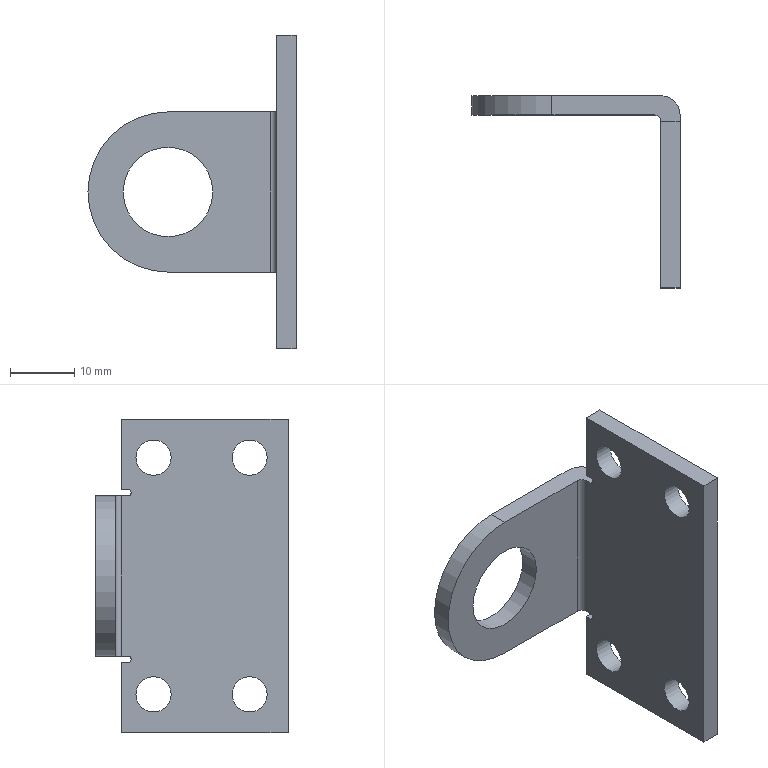Part | NX | features 5003_213_Bracket 2 | 1 solid | 23 faces | box 32.5 x 30 x 49 mm | volume 5335 mm3 | plane 13 | cylinder 10 | commonest cylinder face diameters 5.5 x4 1 x2 2 x1 6 x1 14 x1 25 x1
STEP:
#1=CARTESIAN_POINT('',(-223.775,-557.1,-110.5));
#2=VERTEX_POINT('',#1);
#3=CARTESIAN_POINT('',(-216.775,-557.1,-110.5));
#4=DIRECTION('',(0.,1.,0.));
#5=DIRECTION('',(-1.,0.,0.));
#6=AXIS2_PLACEMENT_3D('',#3,#4,#5);
#7=CIRCLE('',#6,7.);
#8=EDGE_CURVE('',#2,#2,#7,.T.);
#9=ORIENTED_EDGE('',*,*,#8,.T.);
#10=EDGE_LOOP('',(#9));
#11=FACE_BOUND('',#10,.T.);
#12=CARTESIAN_POINT('',(-200.775,-557.1,-123.));
#13=VERTEX_POINT('',#12);
#14=CARTESIAN_POINT('',(-216.775,-557.1,-123.));
#15=VERTEX_POINT('',#14);
#16=CARTESIAN_POINT('',(-216.775,-557.1,-123.));
#17=DIRECTION('',(-1.,0.,0.));
#18=VECTOR('',#17,1000.);
#19=LINE('',#16,#18);
#20=EDGE_CURVE('',#13,#15,#19,.T.);
#21=ORIENTED_EDGE('',*,*,#20,.F.);
#22=CARTESIAN_POINT('',(-200.775,-557.1,-98.));
#23=VERTEX_POINT('',#22);
#24=CARTESIAN_POINT('',(-200.775,-557.1,-98.));
#25=DIRECTION('',(0.,0.,-1.));
#26=VECTOR('',#25,1000.);
#27=LINE('',#24,#26);
#28=EDGE_CURVE('',#13,#23,#27,.F.);
#29=ORIENTED_EDGE('',*,*,#28,.T.);
#30=CARTESIAN_POINT('',(-216.775,-557.1,-98.));
#31=VERTEX_POINT('',#30);
#32=CARTESIAN_POINT('',(-216.775,-557.1,-98.));
#33=DIRECTION('',(1.,0.,0.));
#34=VECTOR('',#33,1000.);
#35=LINE('',#32,#34);
#36=EDGE_CURVE('',#31,#23,#35,.T.);
#37=ORIENTED_EDGE('',*,*,#36,.F.);
#38=CARTESIAN_POINT('',(-216.775,-557.1,-110.5));
#39=DIRECTION('',(0.,1.,0.));
#40=DIRECTION('',(-1.,0.,0.));
#41=AXIS2_PLACEMENT_3D('',#38,#39,#40);
#42=CIRCLE('',#41,12.5);
#43=EDGE_CURVE('',#15,#31,#42,.T.);
#44=ORIENTED_EDGE('',*,*,#43,.F.);
#45=EDGE_LOOP('',(#21,#29,#37,#44));
#46=FACE_BOUND('',#45,.T.);
#47=CARTESIAN_POINT('',(-216.775,-557.1,-110.5));
#48=DIRECTION('',(0.,1.,0.));
#49=DIRECTION('',(-1.,0.,0.));
#50=AXIS2_PLACEMENT_3D('',#47,#48,#49);
#51=PLANE('',#50);
#52=ADVANCED_FACE('',(#11,#46),#51,.F.);
#53=ORIENTED_EDGE('',*,*,#36,.T.);
#54=CARTESIAN_POINT('',(-199.775,-558.1,-98.));
#55=VERTEX_POINT('',#54);
#56=CARTESIAN_POINT('',(-200.775,-558.1,-98.));
#57=DIRECTION('',(0.,0.,-1.));
#58=DIRECTION('',(0.,-1.,0.));
#59=AXIS2_PLACEMENT_3D('',#56,#57,#58);
#60=CIRCLE('',#59,1.);
#61=EDGE_CURVE('',#23,#55,#60,.T.);
#62=ORIENTED_EDGE('',*,*,#61,.T.);
#63=CARTESIAN_POINT('',(-199.775,-559.1,-98.));
#64=VERTEX_POINT('',#63);
#65=CARTESIAN_POINT('',(-199.775,-584.1,-98.));
#66=DIRECTION('',(0.,1.,0.));
#67=VECTOR('',#66,1000.);
#68=LINE('',#65,#67);
#69=EDGE_CURVE('',#64,#55,#68,.T.);
#70=ORIENTED_EDGE('',*,*,#69,.F.);
#71=CARTESIAN_POINT('',(-196.775,-559.1,-98.));
#72=VERTEX_POINT('',#71);
#73=CARTESIAN_POINT('',(-229.275,-559.1,-98.));
#74=DIRECTION('',(1.,0.,0.));
#75=VECTOR('',#74,1000.);
#76=LINE('',#73,#75);
#77=EDGE_CURVE('',#64,#72,#76,.T.);
#78=ORIENTED_EDGE('',*,*,#77,.T.);
#79=CARTESIAN_POINT('',(-196.775,-557.1,-98.));
#80=VERTEX_POINT('',#79);
#81=CARTESIAN_POINT('',(-196.775,-554.1,-98.));
#82=DIRECTION('',(0.,-1.,0.));
#83=VECTOR('',#82,1000.);
#84=LINE('',#81,#83);
#85=EDGE_CURVE('',#80,#72,#84,.T.);
#86=ORIENTED_EDGE('',*,*,#85,.F.);
#87=CARTESIAN_POINT('',(-199.775,-554.1,-98.));
#88=VERTEX_POINT('',#87);
#89=CARTESIAN_POINT('',(-199.775,-557.1,-98.));
#90=DIRECTION('',(0.,0.,-1.));
#91=DIRECTION('',(0.,-1.,0.));
#92=AXIS2_PLACEMENT_3D('',#89,#90,#91);
#93=CIRCLE('',#92,3.);
#94=EDGE_CURVE('',#80,#88,#93,.F.);
#95=ORIENTED_EDGE('',*,*,#94,.T.);
#96=CARTESIAN_POINT('',(-216.775,-554.1,-98.));
#97=VERTEX_POINT('',#96);
#98=CARTESIAN_POINT('',(-216.775,-554.1,-98.));
#99=DIRECTION('',(1.,0.,0.));
#100=VECTOR('',#99,1000.);
#101=LINE('',#98,#100);
#102=EDGE_CURVE('',#97,#88,#101,.T.);
#103=ORIENTED_EDGE('',*,*,#102,.F.);
#104=CARTESIAN_POINT('',(-216.775,-554.1,-98.));
#105=DIRECTION('',(0.,-1.,0.));
#106=VECTOR('',#105,1000.);
#107=LINE('',#104,#106);
#108=EDGE_CURVE('',#97,#31,#107,.T.);
#109=ORIENTED_EDGE('',*,*,#108,.T.);
#110=EDGE_LOOP('',(#53,#62,#70,#78,#86,#95,#103,#109));
#111=FACE_BOUND('',#110,.T.);
#112=CARTESIAN_POINT('',(-216.775,-554.1,-98.));
#113=DIRECTION('',(0.,0.,-1.));
#114=DIRECTION('',(0.,-1.,0.));
#115=AXIS2_PLACEMENT_3D('',#112,#113,#114);
#116=PLANE('',#115);
#117=ADVANCED_FACE('',(#111),#116,.F.);
#118=CARTESIAN_POINT('',(-199.775,-558.1,-123.));
#119=VERTEX_POINT('',#118);
#120=CARTESIAN_POINT('',(-200.775,-558.1,-123.));
#121=DIRECTION('',(0.,0.,1.));
#122=DIRECTION('',(0.,1.,0.));
#123=AXIS2_PLACEMENT_3D('',#120,#121,#122);
#124=CIRCLE('',#123,1.);
#125=EDGE_CURVE('',#119,#13,#124,.T.);
#126=ORIENTED_EDGE('',*,*,#125,.T.);
#127=ORIENTED_EDGE('',*,*,#20,.T.);
#128=CARTESIAN_POINT('',(-216.775,-554.1,-123.));
#129=VERTEX_POINT('',#128);
#130=CARTESIAN_POINT('',(-216.775,-554.1,-123.));
#131=DIRECTION('',(0.,-1.,0.));
#132=VECTOR('',#131,1000.);
#133=LINE('',#130,#132);
#134=EDGE_CURVE('',#129,#15,#133,.T.);
#135=ORIENTED_EDGE('',*,*,#134,.F.);
#136=CARTESIAN_POINT('',(-199.775,-554.1,-123.));
#137=VERTEX_POINT('',#136);
#138=CARTESIAN_POINT('',(-216.775,-554.1,-123.));
#139=DIRECTION('',(-1.,0.,0.));
#140=VECTOR('',#139,1000.);
#141=LINE('',#138,#140);
#142=EDGE_CURVE('',#137,#129,#141,.T.);
#143=ORIENTED_EDGE('',*,*,#142,.F.);
#144=CARTESIAN_POINT('',(-196.775,-557.1,-123.));
#145=VERTEX_POINT('',#144);
#146=CARTESIAN_POINT('',(-199.775,-557.1,-123.));
#147=DIRECTION('',(0.,0.,1.));
#148=DIRECTION('',(0.,1.,0.));
#149=AXIS2_PLACEMENT_3D('',#146,#147,#148);
#150=CIRCLE('',#149,3.);
#151=EDGE_CURVE('',#137,#145,#150,.F.);
#152=ORIENTED_EDGE('',*,*,#151,.T.);
#153=CARTESIAN_POINT('',(-196.775,-559.1,-123.));
#154=VERTEX_POINT('',#153);
#155=CARTESIAN_POINT('',(-196.775,-558.1,-123.));
#156=DIRECTION('',(0.,1.,0.));
#157=VECTOR('',#156,1000.);
#158=LINE('',#155,#157);
#159=EDGE_CURVE('',#154,#145,#158,.T.);
#160=ORIENTED_EDGE('',*,*,#159,.F.);
#161=CARTESIAN_POINT('',(-199.775,-559.1,-123.));
#162=VERTEX_POINT('',#161);
#163=CARTESIAN_POINT('',(-229.275,-559.1,-123.));
#164=DIRECTION('',(1.,0.,0.));
#165=VECTOR('',#164,1000.);
#166=LINE('',#163,#165);
#167=EDGE_CURVE('',#162,#154,#166,.T.);
#168=ORIENTED_EDGE('',*,*,#167,.F.);
#169=CARTESIAN_POINT('',(-199.775,-584.1,-123.));
#170=DIRECTION('',(0.,-1.,0.));
#171=VECTOR('',#170,1000.);
#172=LINE('',#169,#171);
#173=EDGE_CURVE('',#119,#162,#172,.T.);
#174=ORIENTED_EDGE('',*,*,#173,.F.);
#175=EDGE_LOOP('',(#126,#127,#135,#143,#152,#160,#168,#174));
#176=FACE_BOUND('',#175,.T.);
#177=CARTESIAN_POINT('',(-216.775,-554.1,-123.));
#178=DIRECTION('',(0.,0.,1.));
#179=DIRECTION('',(0.,1.,0.));
#180=AXIS2_PLACEMENT_3D('',#177,#178,#179);
#181=PLANE('',#180);
#182=ADVANCED_FACE('',(#176),#181,.F.);
#183=ORIENTED_EDGE('',*,*,#102,.T.);
#184=CARTESIAN_POINT('',(-199.775,-554.1,-123.));
#185=DIRECTION('',(0.,0.,-1.));
#186=VECTOR('',#185,1000.);
#187=LINE('',#184,#186);
#188=EDGE_CURVE('',#88,#137,#187,.T.);
#189=ORIENTED_EDGE('',*,*,#188,.T.);
#190=ORIENTED_EDGE('',*,*,#142,.T.);
#191=CARTESIAN_POINT('',(-216.775,-554.1,-110.5));
#192=DIRECTION('',(0.,1.,0.));
#193=DIRECTION('',(-1.,0.,0.));
#194=AXIS2_PLACEMENT_3D('',#191,#192,#193);
#195=CIRCLE('',#194,12.5);
#196=EDGE_CURVE('',#129,#97,#195,.T.);
#197=ORIENTED_EDGE('',*,*,#196,.T.);
#198=EDGE_LOOP('',(#183,#189,#190,#197));
#199=FACE_BOUND('',#198,.T.);
#200=CARTESIAN_POINT('',(-223.775,-554.1,-110.5));
#201=VERTEX_POINT('',#200);
#202=CARTESIAN_POINT('',(-216.775,-554.1,-110.5));
#203=DIRECTION('',(0.,1.,0.));
#204=DIRECTION('',(-1.,0.,0.));
#205=AXIS2_PLACEMENT_3D('',#202,#203,#204);
#206=CIRCLE('',#205,7.);
#207=EDGE_CURVE('',#201,#201,#206,.T.);
#208=ORIENTED_EDGE('',*,*,#207,.F.);
#209=EDGE_LOOP('',(#208));
#210=FACE_BOUND('',#209,.T.);
#211=CARTESIAN_POINT('',(-216.775,-554.1,-110.5));
#212=DIRECTION('',(0.,1.,0.));
#213=DIRECTION('',(-1.,0.,0.));
#214=AXIS2_PLACEMENT_3D('',#211,#212,#213);
#215=PLANE('',#214);
#216=ADVANCED_FACE('',(#199,#210),#215,.T.);
#217=ORIENTED_EDGE('',*,*,#43,.T.);
#218=ORIENTED_EDGE('',*,*,#108,.F.);
#219=ORIENTED_EDGE('',*,*,#196,.F.);
#220=ORIENTED_EDGE('',*,*,#134,.T.);
#221=EDGE_LOOP('',(#217,#218,#219,#220));
#222=FACE_BOUND('',#221,.T.);
#223=CARTESIAN_POINT('',(-216.775,-554.1,-110.5));
#224=DIRECTION('',(0.,-1.,0.));
#225=DIRECTION('',(1.,0.,0.));
#226=AXIS2_PLACEMENT_3D('',#223,#224,#225);
#227=CYLINDRICAL_SURFACE('',#226,12.5);
#228=ADVANCED_FACE('',(#222),#227,.T.);
#229=CARTESIAN_POINT('',(-196.775,-580.85,-129.));
#230=VERTEX_POINT('',#229);
#231=CARTESIAN_POINT('',(-196.775,-578.1,-129.));
#232=DIRECTION('',(-1.,0.,0.));
#233=DIRECTION('',(0.,-1.,0.));
#234=AXIS2_PLACEMENT_3D('',#231,#232,#233);
#235=CIRCLE('',#234,2.75);
#236=EDGE_CURVE('',#230,#230,#235,.T.);
#237=ORIENTED_EDGE('',*,*,#236,.T.);
#238=EDGE_LOOP('',(#237));
#239=FACE_BOUND('',#238,.T.);
#240=CARTESIAN_POINT('',(-196.775,-565.85,-129.));
#241=VERTEX_POINT('',#240);
#242=CARTESIAN_POINT('',(-196.775,-563.1,-129.));
#243=DIRECTION('',(-1.,0.,0.));
#244=DIRECTION('',(0.,-1.,0.));
#245=AXIS2_PLACEMENT_3D('',#242,#243,#244);
#246=CIRCLE('',#245,2.75);
#247=EDGE_CURVE('',#241,#241,#246,.T.);
#248=ORIENTED_EDGE('',*,*,#247,.T.);
#249=EDGE_LOOP('',(#248));
#250=FACE_BOUND('',#249,.T.);
#251=CARTESIAN_POINT('',(-196.775,-580.85,-92.));
#252=VERTEX_POINT('',#251);
#253=CARTESIAN_POINT('',(-196.775,-578.1,-92.));
#254=DIRECTION('',(-1.,0.,0.));
#255=DIRECTION('',(0.,-1.,0.));
#256=AXIS2_PLACEMENT_3D('',#253,#254,#255);
#257=CIRCLE('',#256,2.75);
#258=EDGE_CURVE('',#252,#252,#257,.T.);
#259=ORIENTED_EDGE('',*,*,#258,.T.);
#260=EDGE_LOOP('',(#259));
#261=FACE_BOUND('',#260,.T.);
#262=CARTESIAN_POINT('',(-196.775,-565.85,-92.));
#263=VERTEX_POINT('',#262);
#264=CARTESIAN_POINT('',(-196.775,-563.1,-92.));
#265=DIRECTION('',(-1.,0.,0.));
#266=DIRECTION('',(0.,-1.,0.));
#267=AXIS2_PLACEMENT_3D('',#264,#265,#266);
#268=CIRCLE('',#267,2.75);
#269=EDGE_CURVE('',#263,#263,#268,.T.);
#270=ORIENTED_EDGE('',*,*,#269,.T.);
#271=EDGE_LOOP('',(#270));
#272=FACE_BOUND('',#271,.T.);
#273=ORIENTED_EDGE('',*,*,#85,.T.);
#274=CARTESIAN_POINT('',(-196.775,-559.1,-97.));
#275=VERTEX_POINT('',#274);
#276=CARTESIAN_POINT('',(-196.775,-559.1,-97.5));
#277=DIRECTION('',(1.,0.,0.));
#278=DIRECTION('',(0.,1.,0.));
#279=AXIS2_PLACEMENT_3D('',#276,#277,#278);
#280=CIRCLE('',#279,0.5);
#281=EDGE_CURVE('',#275,#72,#280,.T.);
#282=ORIENTED_EDGE('',*,*,#281,.F.);
#283=CARTESIAN_POINT('',(-196.775,-558.1,-97.));
#284=VERTEX_POINT('',#283);
#285=CARTESIAN_POINT('',(-196.775,-557.1,-97.));
#286=DIRECTION('',(0.,-1.,0.));
#287=VECTOR('',#286,1000.);
#288=LINE('',#285,#287);
#289=EDGE_CURVE('',#284,#275,#288,.T.);
#290=ORIENTED_EDGE('',*,*,#289,.F.);
#291=CARTESIAN_POINT('',(-196.775,-558.1,-86.));
#292=VERTEX_POINT('',#291);
#293=CARTESIAN_POINT('',(-196.775,-558.1,-86.));
#294=DIRECTION('',(0.,0.,1.));
#295=VECTOR('',#294,1000.);
#296=LINE('',#293,#295);
#297=EDGE_CURVE('',#284,#292,#296,.T.);
#298=ORIENTED_EDGE('',*,*,#297,.T.);
#299=CARTESIAN_POINT('',(-196.775,-584.1,-86.));
#300=VERTEX_POINT('',#299);
#301=CARTESIAN_POINT('',(-196.775,-584.1,-86.));
#302=DIRECTION('',(0.,1.,0.));
#303=VECTOR('',#302,1000.);
#304=LINE('',#301,#303);
#305=EDGE_CURVE('',#300,#292,#304,.T.);
#306=ORIENTED_EDGE('',*,*,#305,.F.);
#307=CARTESIAN_POINT('',(-196.775,-584.1,-135.));
#308=VERTEX_POINT('',#307);
#309=CARTESIAN_POINT('',(-196.775,-584.1,-135.));
#310=DIRECTION('',(0.,0.,1.));
#311=VECTOR('',#310,1000.);
#312=LINE('',#309,#311);
#313=EDGE_CURVE('',#308,#300,#312,.T.);
#314=ORIENTED_EDGE('',*,*,#313,.F.);
#315=CARTESIAN_POINT('',(-196.775,-558.1,-135.));
#316=VERTEX_POINT('',#315);
#317=CARTESIAN_POINT('',(-196.775,-584.1,-135.));
#318=DIRECTION('',(0.,1.,0.));
#319=VECTOR('',#318,1000.);
#320=LINE('',#317,#319);
#321=EDGE_CURVE('',#308,#316,#320,.T.);
#322=ORIENTED_EDGE('',*,*,#321,.T.);
#323=CARTESIAN_POINT('',(-196.775,-558.1,-124.));
#324=VERTEX_POINT('',#323);
#325=CARTESIAN_POINT('',(-196.775,-558.1,-123.));
#326=DIRECTION('',(0.,0.,1.));
#327=VECTOR('',#326,1000.);
#328=LINE('',#325,#327);
#329=EDGE_CURVE('',#316,#324,#328,.T.);
#330=ORIENTED_EDGE('',*,*,#329,.T.);
#331=CARTESIAN_POINT('',(-196.775,-559.1,-124.));
#332=VERTEX_POINT('',#331);
#333=CARTESIAN_POINT('',(-196.775,-557.1,-124.));
#334=DIRECTION('',(0.,1.,0.));
#335=VECTOR('',#334,1000.);
#336=LINE('',#333,#335);
#337=EDGE_CURVE('',#332,#324,#336,.T.);
#338=ORIENTED_EDGE('',*,*,#337,.F.);
#339=CARTESIAN_POINT('',(-196.775,-559.1,-123.5));
#340=DIRECTION('',(1.,0.,0.));
#341=DIRECTION('',(0.,-1.,0.));
#342=AXIS2_PLACEMENT_3D('',#339,#340,#341);
#343=CIRCLE('',#342,0.5);
#344=EDGE_CURVE('',#154,#332,#343,.T.);
#345=ORIENTED_EDGE('',*,*,#344,.F.);
#346=ORIENTED_EDGE('',*,*,#159,.T.);
#347=CARTESIAN_POINT('',(-196.775,-557.1,-98.));
#348=DIRECTION('',(0.,0.,-1.));
#349=VECTOR('',#348,1000.);
#350=LINE('',#347,#349);
#351=EDGE_CURVE('',#145,#80,#350,.F.);
#352=ORIENTED_EDGE('',*,*,#351,.T.);
#353=EDGE_LOOP('',(#273,#282,#290,#298,#306,#314,#322,#330,#338,#345,#346,#352));
#354=FACE_BOUND('',#353,.T.);
#355=CARTESIAN_POINT('',(-196.775,-554.1,-123.));
#356=DIRECTION('',(-1.,0.,0.));
#357=DIRECTION('',(0.,-1.,0.));
#358=AXIS2_PLACEMENT_3D('',#355,#356,#357);
#359=PLANE('',#358);
#360=ADVANCED_FACE('',(#239,#250,#261,#272,#354),#359,.F.);
#361=ORIENTED_EDGE('',*,*,#207,.T.);
#362=EDGE_LOOP('',(#361));
#363=FACE_BOUND('',#362,.T.);
#364=ORIENTED_EDGE('',*,*,#8,.F.);
#365=EDGE_LOOP('',(#364));
#366=FACE_BOUND('',#365,.T.);
#367=CARTESIAN_POINT('',(-216.775,-554.1,-110.5));
#368=DIRECTION('',(0.,-1.,0.));
#369=DIRECTION('',(1.,0.,0.));
#370=AXIS2_PLACEMENT_3D('',#367,#368,#369);
#371=CYLINDRICAL_SURFACE('',#370,7.);
#372=ADVANCED_FACE('',(#363,#366),#371,.F.);
#373=CARTESIAN_POINT('',(-199.775,-580.85,-129.));
#374=VERTEX_POINT('',#373);
#375=CARTESIAN_POINT('',(-199.775,-578.1,-129.));
#376=DIRECTION('',(-1.,0.,0.));
#377=DIRECTION('',(0.,-1.,0.));
#378=AXIS2_PLACEMENT_3D('',#375,#376,#377);
#379=CIRCLE('',#378,2.75);
#380=EDGE_CURVE('',#374,#374,#379,.T.);
#381=ORIENTED_EDGE('',*,*,#380,.F.);
#382=EDGE_LOOP('',(#381));
#383=FACE_BOUND('',#382,.T.);
#384=CARTESIAN_POINT('',(-199.775,-565.85,-129.));
#385=VERTEX_POINT('',#384);
#386=CARTESIAN_POINT('',(-199.775,-563.1,-129.));
#387=DIRECTION('',(-1.,0.,0.));
#388=DIRECTION('',(0.,-1.,0.));
#389=AXIS2_PLACEMENT_3D('',#386,#387,#388);
#390=CIRCLE('',#389,2.75);
#391=EDGE_CURVE('',#385,#385,#390,.T.);
#392=ORIENTED_EDGE('',*,*,#391,.F.);
#393=EDGE_LOOP('',(#392));
#394=FACE_BOUND('',#393,.T.);
#395=CARTESIAN_POINT('',(-199.775,-580.85,-92.));
#396=VERTEX_POINT('',#395);
#397=CARTESIAN_POINT('',(-199.775,-578.1,-92.));
#398=DIRECTION('',(-1.,0.,0.));
#399=DIRECTION('',(0.,-1.,0.));
#400=AXIS2_PLACEMENT_3D('',#397,#398,#399);
#401=CIRCLE('',#400,2.75);
#402=EDGE_CURVE('',#396,#396,#401,.T.);
#403=ORIENTED_EDGE('',*,*,#402,.F.);
#404=EDGE_LOOP('',(#403));
#405=FACE_BOUND('',#404,.T.);
#406=CARTESIAN_POINT('',(-199.775,-565.85,-92.));
#407=VERTEX_POINT('',#406);
#408=CARTESIAN_POINT('',(-199.775,-563.1,-92.));
#409=DIRECTION('',(-1.,0.,0.));
#410=DIRECTION('',(0.,-1.,0.));
#411=AXIS2_PLACEMENT_3D('',#408,#409,#410);
#412=CIRCLE('',#411,2.75);
#413=EDGE_CURVE('',#407,#407,#412,.T.);
#414=ORIENTED_EDGE('',*,*,#413,.F.);
#415=EDGE_LOOP('',(#414));
#416=FACE_BOUND('',#415,.T.);
#417=CARTESIAN_POINT('',(-199.775,-559.1,-97.));
#418=VERTEX_POINT('',#417);
#419=CARTESIAN_POINT('',(-199.775,-559.1,-97.5));
#420=DIRECTION('',(1.,0.,0.));
#421=DIRECTION('',(0.,1.,0.));
#422=AXIS2_PLACEMENT_3D('',#419,#420,#421);
#423=CIRCLE('',#422,0.5);
#424=EDGE_CURVE('',#418,#64,#423,.T.);
#425=ORIENTED_EDGE('',*,*,#424,.T.);
#426=ORIENTED_EDGE('',*,*,#69,.T.);
#427=CARTESIAN_POINT('',(-199.775,-558.1,-123.));
#428=DIRECTION('',(0.,0.,-1.));
#429=VECTOR('',#428,1000.);
#430=LINE('',#427,#429);
#431=EDGE_CURVE('',#55,#119,#430,.T.);
#432=ORIENTED_EDGE('',*,*,#431,.T.);
#433=ORIENTED_EDGE('',*,*,#173,.T.);
#434=CARTESIAN_POINT('',(-199.775,-559.1,-124.));
#435=VERTEX_POINT('',#434);
#436=CARTESIAN_POINT('',(-199.775,-559.1,-123.5));
#437=DIRECTION('',(1.,0.,0.));
#438=DIRECTION('',(0.,1.,0.));
#439=AXIS2_PLACEMENT_3D('',#436,#437,#438);
#440=CIRCLE('',#439,0.5);
#441=EDGE_CURVE('',#162,#435,#440,.T.);
#442=ORIENTED_EDGE('',*,*,#441,.T.);
#443=CARTESIAN_POINT('',(-199.775,-558.1,-124.));
#444=VERTEX_POINT('',#443);
#445=CARTESIAN_POINT('',(-199.775,-584.1,-124.));
#446=DIRECTION('',(0.,1.,0.));
#447=VECTOR('',#446,1000.);
#448=LINE('',#445,#447);
#449=EDGE_CURVE('',#435,#444,#448,.T.);
#450=ORIENTED_EDGE('',*,*,#449,.T.);
#451=CARTESIAN_POINT('',(-199.775,-558.1,-135.));
#452=VERTEX_POINT('',#451);
#453=CARTESIAN_POINT('',(-199.775,-558.1,-123.));
#454=DIRECTION('',(0.,0.,1.));
#455=VECTOR('',#454,1000.);
#456=LINE('',#453,#455);
#457=EDGE_CURVE('',#452,#444,#456,.T.);
#458=ORIENTED_EDGE('',*,*,#457,.F.);
#459=CARTESIAN_POINT('',(-199.775,-584.1,-135.));
#460=VERTEX_POINT('',#459);
#461=CARTESIAN_POINT('',(-199.775,-584.1,-135.));
#462=DIRECTION('',(0.,1.,0.));
#463=VECTOR('',#462,1000.);
#464=LINE('',#461,#463);
#465=EDGE_CURVE('',#460,#452,#464,.T.);
#466=ORIENTED_EDGE('',*,*,#465,.F.);
#467=CARTESIAN_POINT('',(-199.775,-584.1,-86.));
#468=VERTEX_POINT('',#467);
#469=CARTESIAN_POINT('',(-199.775,-584.1,-135.));
#470=DIRECTION('',(0.,0.,-1.));
#471=VECTOR('',#470,1000.);
#472=LINE('',#469,#471);
#473=EDGE_CURVE('',#468,#460,#472,.T.);
#474=ORIENTED_EDGE('',*,*,#473,.F.);
#475=CARTESIAN_POINT('',(-199.775,-558.1,-86.));
#476=VERTEX_POINT('',#475);
#477=CARTESIAN_POINT('',(-199.775,-584.1,-86.));
#478=DIRECTION('',(0.,1.,0.));
#479=VECTOR('',#478,1000.);
#480=LINE('',#477,#479);
#481=EDGE_CURVE('',#468,#476,#480,.T.);
#482=ORIENTED_EDGE('',*,*,#481,.T.);
#483=CARTESIAN_POINT('',(-199.775,-558.1,-97.));
#484=VERTEX_POINT('',#483);
#485=CARTESIAN_POINT('',(-199.775,-558.1,-86.));
#486=DIRECTION('',(0.,0.,1.));
#487=VECTOR('',#486,1000.);
#488=LINE('',#485,#487);
#489=EDGE_CURVE('',#484,#476,#488,.T.);
#490=ORIENTED_EDGE('',*,*,#489,.F.);
#491=CARTESIAN_POINT('',(-199.775,-584.1,-97.));
#492=DIRECTION('',(0.,-1.,0.));
#493=VECTOR('',#492,1000.);
#494=LINE('',#491,#493);
#495=EDGE_CURVE('',#484,#418,#494,.T.);
#496=ORIENTED_EDGE('',*,*,#495,.T.);
#497=EDGE_LOOP('',(#425,#426,#432,#433,#442,#450,#458,#466,#474,#482,#490,#496));
#498=FACE_BOUND('',#497,.T.);
#499=CARTESIAN_POINT('',(-199.775,-584.1,-135.));
#500=DIRECTION('',(1.,0.,0.));
#501=DIRECTION('',(0.,1.,0.));
#502=AXIS2_PLACEMENT_3D('',#499,#500,#501);
#503=PLANE('',#502);
#504=ADVANCED_FACE('',(#383,#394,#405,#416,#498),#503,.F.);
#505=ORIENTED_EDGE('',*,*,#305,.T.);
#506=CARTESIAN_POINT('',(-196.775,-558.1,-86.));
#507=DIRECTION('',(-1.,0.,0.));
#508=VECTOR('',#507,1000.);
#509=LINE('',#506,#508);
#510=EDGE_CURVE('',#292,#476,#509,.T.);
#511=ORIENTED_EDGE('',*,*,#510,.T.);
#512=ORIENTED_EDGE('',*,*,#481,.F.);
#513=CARTESIAN_POINT('',(-196.775,-584.1,-86.));
#514=DIRECTION('',(-1.,0.,0.));
#515=VECTOR('',#514,1000.);
#516=LINE('',#513,#515);
#517=EDGE_CURVE('',#300,#468,#516,.T.);
#518=ORIENTED_EDGE('',*,*,#517,.F.);
#519=EDGE_LOOP('',(#505,#511,#512,#518));
#520=FACE_BOUND('',#519,.T.);
#521=CARTESIAN_POINT('',(-196.775,-584.1,-86.));
#522=DIRECTION('',(0.,0.,-1.));
#523=DIRECTION('',(0.,-1.,0.));
#524=AXIS2_PLACEMENT_3D('',#521,#522,#523);
#525=PLANE('',#524);
#526=ADVANCED_FACE('',(#520),#525,.F.);
#527=ORIENTED_EDGE('',*,*,#465,.T.);
#528=CARTESIAN_POINT('',(-196.775,-558.1,-135.));
#529=DIRECTION('',(-1.,0.,0.));
#530=VECTOR('',#529,1000.);
#531=LINE('',#528,#530);
#532=EDGE_CURVE('',#316,#452,#531,.T.);
#533=ORIENTED_EDGE('',*,*,#532,.F.);
#534=ORIENTED_EDGE('',*,*,#321,.F.);
#535=CARTESIAN_POINT('',(-196.775,-584.1,-135.));
#536=DIRECTION('',(1.,0.,0.));
#537=VECTOR('',#536,1000.);
#538=LINE('',#535,#537);
#539=EDGE_CURVE('',#460,#308,#538,.T.);
#540=ORIENTED_EDGE('',*,*,#539,.F.);
#541=EDGE_LOOP('',(#527,#533,#534,#540));
#542=FACE_BOUND('',#541,.T.);
#543=CARTESIAN_POINT('',(-196.775,-584.1,-135.));
#544=DIRECTION('',(0.,0.,1.));
#545=DIRECTION('',(0.,1.,0.));
#546=AXIS2_PLACEMENT_3D('',#543,#544,#545);
#547=PLANE('',#546);
#548=ADVANCED_FACE('',(#542),#547,.F.);
#549=ORIENTED_EDGE('',*,*,#313,.T.);
#550=ORIENTED_EDGE('',*,*,#517,.T.);
#551=ORIENTED_EDGE('',*,*,#473,.T.);
#552=ORIENTED_EDGE('',*,*,#539,.T.);
#553=EDGE_LOOP('',(#549,#550,#551,#552));
#554=FACE_BOUND('',#553,.T.);
#555=CARTESIAN_POINT('',(-38.31,-584.1,-228.));
#556=DIRECTION('',(0.,-1.,0.));
#557=DIRECTION('',(1.,0.,0.));
#558=AXIS2_PLACEMENT_3D('',#555,#556,#557);
#559=PLANE('',#558);
#560=ADVANCED_FACE('',(#554),#559,.T.);
#561=ORIENTED_EDGE('',*,*,#61,.F.);
#562=ORIENTED_EDGE('',*,*,#28,.F.);
#563=ORIENTED_EDGE('',*,*,#125,.F.);
#564=ORIENTED_EDGE('',*,*,#431,.F.);
#565=EDGE_LOOP('',(#561,#562,#563,#564));
#566=FACE_BOUND('',#565,.T.);
#567=CARTESIAN_POINT('',(-200.775,-558.1,-135.));
#568=DIRECTION('',(0.,0.,1.));
#569=DIRECTION('',(0.,1.,0.));
#570=AXIS2_PLACEMENT_3D('',#567,#568,#569);
#571=CYLINDRICAL_SURFACE('',#570,1.);
#572=ADVANCED_FACE('',(#566),#571,.F.);
#573=ORIENTED_EDGE('',*,*,#457,.T.);
#574=CARTESIAN_POINT('',(-196.775,-558.1,-124.));
#575=DIRECTION('',(1.,0.,0.));
#576=VECTOR('',#575,1000.);
#577=LINE('',#574,#576);
#578=EDGE_CURVE('',#444,#324,#577,.T.);
#579=ORIENTED_EDGE('',*,*,#578,.T.);
#580=ORIENTED_EDGE('',*,*,#329,.F.);
#581=ORIENTED_EDGE('',*,*,#532,.T.);
#582=EDGE_LOOP('',(#573,#579,#580,#581));
#583=FACE_BOUND('',#582,.T.);
#584=CARTESIAN_POINT('',(-196.775,-558.1,-123.));
#585=DIRECTION('',(0.,-1.,0.));
#586=DIRECTION('',(0.,0.,1.));
#587=AXIS2_PLACEMENT_3D('',#584,#585,#586);
#588=PLANE('',#587);
#589=ADVANCED_FACE('',(#583),#588,.F.);
#590=ORIENTED_EDGE('',*,*,#297,.F.);
#591=CARTESIAN_POINT('',(-196.775,-558.1,-97.));
#592=DIRECTION('',(-1.,0.,0.));
#593=VECTOR('',#592,1000.);
#594=LINE('',#591,#593);
#595=EDGE_CURVE('',#284,#484,#594,.T.);
#596=ORIENTED_EDGE('',*,*,#595,.T.);
#597=ORIENTED_EDGE('',*,*,#489,.T.);
#598=ORIENTED_EDGE('',*,*,#510,.F.);
#599=EDGE_LOOP('',(#590,#596,#597,#598));
#600=FACE_BOUND('',#599,.T.);
#601=CARTESIAN_POINT('',(-196.775,-558.1,-86.));
#602=DIRECTION('',(0.,-1.,0.));
#603=DIRECTION('',(0.,0.,1.));
#604=AXIS2_PLACEMENT_3D('',#601,#602,#603);
#605=PLANE('',#604);
#606=ADVANCED_FACE('',(#600),#605,.F.);
#607=ORIENTED_EDGE('',*,*,#269,.F.);
#608=EDGE_LOOP('',(#607));
#609=FACE_BOUND('',#608,.T.);
#610=ORIENTED_EDGE('',*,*,#413,.T.);
#611=EDGE_LOOP('',(#610));
#612=FACE_BOUND('',#611,.T.);
#613=CARTESIAN_POINT('',(-196.775,-563.1,-92.));
#614=DIRECTION('',(-1.,0.,0.));
#615=DIRECTION('',(0.,-1.,0.));
#616=AXIS2_PLACEMENT_3D('',#613,#614,#615);
#617=CYLINDRICAL_SURFACE('',#616,2.75);
#618=ADVANCED_FACE('',(#609,#612),#617,.F.);
#619=ORIENTED_EDGE('',*,*,#258,.F.);
#620=EDGE_LOOP('',(#619));
#621=FACE_BOUND('',#620,.T.);
#622=ORIENTED_EDGE('',*,*,#402,.T.);
#623=EDGE_LOOP('',(#622));
#624=FACE_BOUND('',#623,.T.);
#625=CARTESIAN_POINT('',(-196.775,-578.1,-92.));
#626=DIRECTION('',(-1.,0.,0.));
#627=DIRECTION('',(0.,-1.,0.));
#628=AXIS2_PLACEMENT_3D('',#625,#626,#627);
#629=CYLINDRICAL_SURFACE('',#628,2.75);
#630=ADVANCED_FACE('',(#621,#624),#629,.F.);
#631=ORIENTED_EDGE('',*,*,#247,.F.);
#632=EDGE_LOOP('',(#631));
#633=FACE_BOUND('',#632,.T.);
#634=ORIENTED_EDGE('',*,*,#391,.T.);
#635=EDGE_LOOP('',(#634));
#636=FACE_BOUND('',#635,.T.);
#637=CARTESIAN_POINT('',(-196.775,-563.1,-129.));
#638=DIRECTION('',(-1.,0.,0.));
#639=DIRECTION('',(0.,-1.,0.));
#640=AXIS2_PLACEMENT_3D('',#637,#638,#639);
#641=CYLINDRICAL_SURFACE('',#640,2.75);
#642=ADVANCED_FACE('',(#633,#636),#641,.F.);
#643=ORIENTED_EDGE('',*,*,#236,.F.);
#644=EDGE_LOOP('',(#643));
#645=FACE_BOUND('',#644,.T.);
#646=ORIENTED_EDGE('',*,*,#380,.T.);
#647=EDGE_LOOP('',(#646));
#648=FACE_BOUND('',#647,.T.);
#649=CARTESIAN_POINT('',(-196.775,-578.1,-129.));
#650=DIRECTION('',(-1.,0.,0.));
#651=DIRECTION('',(0.,-1.,0.));
#652=AXIS2_PLACEMENT_3D('',#649,#650,#651);
#653=CYLINDRICAL_SURFACE('',#652,2.75);
#654=ADVANCED_FACE('',(#645,#648),#653,.F.);
#655=ORIENTED_EDGE('',*,*,#94,.F.);
#656=ORIENTED_EDGE('',*,*,#351,.F.);
#657=ORIENTED_EDGE('',*,*,#151,.F.);
#658=ORIENTED_EDGE('',*,*,#188,.F.);
#659=EDGE_LOOP('',(#655,#656,#657,#658));
#660=FACE_BOUND('',#659,.T.);
#661=CARTESIAN_POINT('',(-199.775,-557.1,-110.5));
#662=DIRECTION('',(0.,0.,1.));
#663=DIRECTION('',(0.,1.,0.));
#664=AXIS2_PLACEMENT_3D('',#661,#662,#663);
#665=CYLINDRICAL_SURFACE('',#664,3.);
#666=ADVANCED_FACE('',(#660),#665,.T.);
#667=CARTESIAN_POINT('',(-229.275,-559.1,-97.));
#668=DIRECTION('',(1.,0.,0.));
#669=VECTOR('',#668,1000.);
#670=LINE('',#667,#669);
#671=EDGE_CURVE('',#418,#275,#670,.T.);
#672=ORIENTED_EDGE('',*,*,#671,.T.);
#673=ORIENTED_EDGE('',*,*,#281,.T.);
#674=ORIENTED_EDGE('',*,*,#77,.F.);
#675=ORIENTED_EDGE('',*,*,#424,.F.);
#676=EDGE_LOOP('',(#672,#673,#674,#675));
#677=FACE_BOUND('',#676,.T.);
#678=CARTESIAN_POINT('',(-229.275,-559.1,-97.5));
#679=DIRECTION('',(1.,0.,0.));
#680=DIRECTION('',(0.,1.,0.));
#681=AXIS2_PLACEMENT_3D('',#678,#679,#680);
#682=CYLINDRICAL_SURFACE('',#681,0.5);
#683=ADVANCED_FACE('',(#677),#682,.F.);
#684=ORIENTED_EDGE('',*,*,#595,.F.);
#685=ORIENTED_EDGE('',*,*,#289,.T.);
#686=ORIENTED_EDGE('',*,*,#671,.F.);
#687=ORIENTED_EDGE('',*,*,#495,.F.);
#688=EDGE_LOOP('',(#684,#685,#686,#687));
#689=FACE_BOUND('',#688,.T.);
#690=CARTESIAN_POINT('',(-229.275,-557.1,-97.));
#691=DIRECTION('',(0.,0.,1.));
#692=DIRECTION('',(0.,1.,0.));
#693=AXIS2_PLACEMENT_3D('',#690,#691,#692);
#694=PLANE('',#693);
#695=ADVANCED_FACE('',(#689),#694,.F.);
#696=ORIENTED_EDGE('',*,*,#167,.T.);
#697=ORIENTED_EDGE('',*,*,#344,.T.);
#698=CARTESIAN_POINT('',(-229.275,-559.1,-124.));
#699=DIRECTION('',(1.,0.,0.));
#700=VECTOR('',#699,1000.);
#701=LINE('',#698,#700);
#702=EDGE_CURVE('',#435,#332,#701,.T.);
#703=ORIENTED_EDGE('',*,*,#702,.F.);
#704=ORIENTED_EDGE('',*,*,#441,.F.);
#705=EDGE_LOOP('',(#696,#697,#703,#704));
#706=FACE_BOUND('',#705,.T.);
#707=CARTESIAN_POINT('',(-229.275,-559.1,-123.5));
#708=DIRECTION('',(1.,0.,0.));
#709=DIRECTION('',(0.,1.,0.));
#710=AXIS2_PLACEMENT_3D('',#707,#708,#709);
#711=CYLINDRICAL_SURFACE('',#710,0.5);
#712=ADVANCED_FACE('',(#706),#711,.F.);
#713=ORIENTED_EDGE('',*,*,#702,.T.);
#714=ORIENTED_EDGE('',*,*,#337,.T.);
#715=ORIENTED_EDGE('',*,*,#578,.F.);
#716=ORIENTED_EDGE('',*,*,#449,.F.);
#717=EDGE_LOOP('',(#713,#714,#715,#716));
#718=FACE_BOUND('',#717,.T.);
#719=CARTESIAN_POINT('',(-229.275,-557.1,-124.));
#720=DIRECTION('',(0.,0.,-1.));
#721=DIRECTION('',(0.,-1.,0.));
#722=AXIS2_PLACEMENT_3D('',#719,#720,#721);
#723=PLANE('',#722);
#724=ADVANCED_FACE('',(#718),#723,.F.);
#725=CLOSED_SHELL('',(#52,#117,#182,#216,#228,#360,#372,#504,#526,#548,#560,#572,#589,#606,#618,#630,#642,#654,#666,#683,#695,#712,#724));
#726=MANIFOLD_SOLID_BREP('',#725);
#727=(LENGTH_UNIT()NAMED_UNIT(*)SI_UNIT(.MILLI.,.METRE.));
#728=UNCERTAINTY_MEASURE_WITH_UNIT(LENGTH_MEASURE(0.00001),#727,'','');
#729=(NAMED_UNIT(*)PLANE_ANGLE_UNIT()SI_UNIT($,.RADIAN.));
#730=(NAMED_UNIT(*)SI_UNIT($,.STERADIAN.)SOLID_ANGLE_UNIT());
#731=(GEOMETRIC_REPRESENTATION_CONTEXT(3)GLOBAL_UNCERTAINTY_ASSIGNED_CONTEXT((#728))GLOBAL_UNIT_ASSIGNED_CONTEXT((#727,#729,#730))REPRESENTATION_CONTEXT('',''));
#732=ADVANCED_BREP_SHAPE_REPRESENTATION('',(#726),#731);